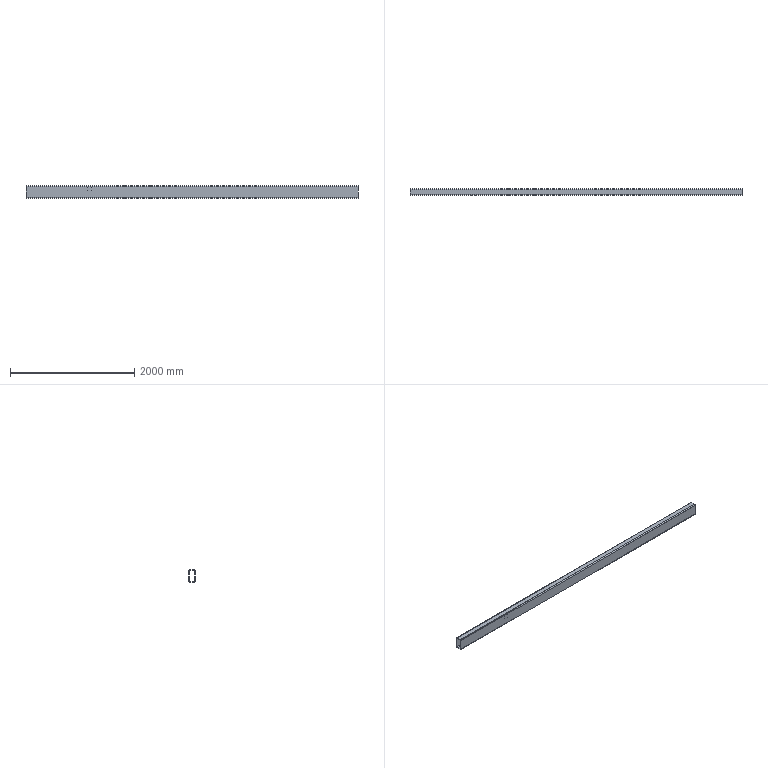Part | STEP file | 1 solid | 26 faces | box 5334 x 100 x 200 mm | volume 23358303 mm3 | cylinder 16 | plane 10 | commonest cylinder face diameters 3.3 x8 16 x4 32 x4